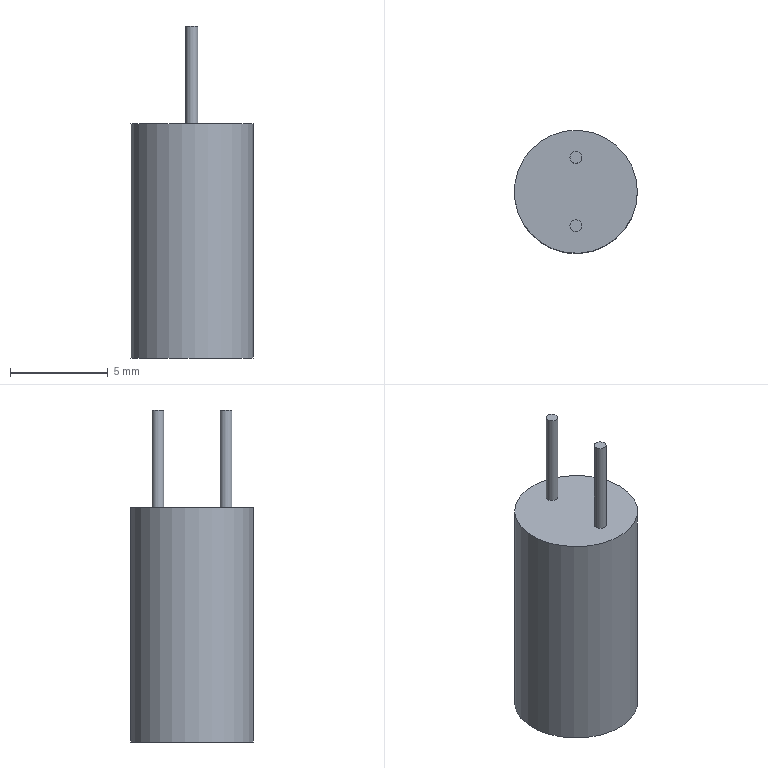Part | STEP file | 118EC225 capacitor | 1 solid | 7 faces | box 6.3 x 6.3 x 17 mm | volume 376.897 mm3 | plane 4 | cylinder 3 | commonest cylinder face diameters 0.6 x2 6.3 x1
STEP:
#1=CARTESIAN_POINT('',(0.,0.,0.));
#2=DIRECTION('',(0.,0.,1.));
#3=DIRECTION('',(1.,0.,0.));
#4=AXIS2_PLACEMENT_3D('',#1,#2,#3);
#5=CARTESIAN_POINT('',(868.15,918.,12.));
#6=VERTEX_POINT('',#5);
#7=CARTESIAN_POINT('',(865.,918.,12.));
#8=DIRECTION('',(0.,0.,1.));
#9=DIRECTION('',(1.,0.,0.));
#10=AXIS2_PLACEMENT_3D('',#7,#8,#9);
#11=CIRCLE('',#10,3.15);
#12=CARTESIAN_POINT('',(865.,918.,12.));
#13=DIRECTION('',(0.,0.,-1.));
#14=DIRECTION('',(-1.,0.,0.));
#15=AXIS2_PLACEMENT_3D('',#12,#13,#14);
#16=CYLINDRICAL_SURFACE('',#15,3.15);
#17=CARTESIAN_POINT('',(9.425,0.));
#18=DIRECTION('',(-1.,0.));
#19=VECTOR('',#18,1.);
#20=LINE('',#17,#19);
#21=(GEOMETRIC_REPRESENTATION_CONTEXT(2)PARAMETRIC_REPRESENTATION_CONTEXT()REPRESENTATION_CONTEXT('',''));
#22=DEFINITIONAL_REPRESENTATION('',(#20),#21);
#23=PCURVE('',#16,#22);
#24=CARTESIAN_POINT('',(865.,918.,12.));
#25=DIRECTION('',(0.,0.,1.));
#26=DIRECTION('',(1.,0.,0.));
#27=AXIS2_PLACEMENT_3D('',#24,#25,#26);
#28=PLANE('',#27);
#29=CARTESIAN_POINT('',(0.,0.));
#30=DIRECTION('',(1.,0.));
#31=AXIS2_PLACEMENT_2D('',#29,#30);
#32=CIRCLE('',#31,3.15);
#33=(GEOMETRIC_REPRESENTATION_CONTEXT(2)PARAMETRIC_REPRESENTATION_CONTEXT()REPRESENTATION_CONTEXT('',''));
#34=DEFINITIONAL_REPRESENTATION('',(#32),#33);
#35=PCURVE('',#28,#34);
#36=SURFACE_CURVE('',#11,(#23,#35),.PCURVE_S1.);
#37=EDGE_CURVE('',#6,#6,#36,.T.);
#38=ORIENTED_EDGE('',*,*,#37,.F.);
#39=CARTESIAN_POINT('',(868.15,918.,0.));
#40=VERTEX_POINT('',#39);
#41=CARTESIAN_POINT('',(868.15,918.,12.));
#42=CARTESIAN_POINT('',(868.15,918.,0.));
#43=B_SPLINE_CURVE_WITH_KNOTS('',1,(#41,#42),.UNSPECIFIED.,.F.,.F.,(2,2),(0.,12.),.PIECEWISE_BEZIER_KNOTS.);
#44=CARTESIAN_POINT('',(9.425,0.));
#45=DIRECTION('',(0.,1.));
#46=VECTOR('',#45,1.);
#47=LINE('',#44,#46);
#48=(GEOMETRIC_REPRESENTATION_CONTEXT(2)PARAMETRIC_REPRESENTATION_CONTEXT()REPRESENTATION_CONTEXT('',''));
#49=DEFINITIONAL_REPRESENTATION('',(#47),#48);
#50=PCURVE('',#16,#49);
#51=CARTESIAN_POINT('',(3.142,0.));
#52=DIRECTION('',(0.,1.));
#53=VECTOR('',#52,1.);
#54=LINE('',#51,#53);
#55=(GEOMETRIC_REPRESENTATION_CONTEXT(2)PARAMETRIC_REPRESENTATION_CONTEXT()REPRESENTATION_CONTEXT('',''));
#56=DEFINITIONAL_REPRESENTATION('',(#54),#55);
#57=PCURVE('',#16,#56);
#58=SEAM_CURVE('',#43,(#50,#57),.PCURVE_S1.);
#59=EDGE_CURVE('',#6,#40,#58,.T.);
#60=ORIENTED_EDGE('',*,*,#59,.T.);
#61=CARTESIAN_POINT('',(865.,918.,0.));
#62=DIRECTION('',(0.,0.,1.));
#63=DIRECTION('',(1.,0.,0.));
#64=AXIS2_PLACEMENT_3D('',#61,#62,#63);
#65=CIRCLE('',#64,3.15);
#66=CARTESIAN_POINT('',(9.425,12.));
#67=DIRECTION('',(-1.,0.));
#68=VECTOR('',#67,1.);
#69=LINE('',#66,#68);
#70=(GEOMETRIC_REPRESENTATION_CONTEXT(2)PARAMETRIC_REPRESENTATION_CONTEXT()REPRESENTATION_CONTEXT('',''));
#71=DEFINITIONAL_REPRESENTATION('',(#69),#70);
#72=PCURVE('',#16,#71);
#73=CARTESIAN_POINT('',(865.,918.,0.));
#74=DIRECTION('',(0.,0.,1.));
#75=DIRECTION('',(1.,0.,0.));
#76=AXIS2_PLACEMENT_3D('',#73,#74,#75);
#77=PLANE('',#76);
#78=CARTESIAN_POINT('',(0.,0.));
#79=DIRECTION('',(1.,0.));
#80=AXIS2_PLACEMENT_2D('',#78,#79);
#81=CIRCLE('',#80,3.15);
#82=(GEOMETRIC_REPRESENTATION_CONTEXT(2)PARAMETRIC_REPRESENTATION_CONTEXT()REPRESENTATION_CONTEXT('',''));
#83=DEFINITIONAL_REPRESENTATION('',(#81),#82);
#84=PCURVE('',#77,#83);
#85=SURFACE_CURVE('',#65,(#72,#84),.PCURVE_S1.);
#86=EDGE_CURVE('',#40,#40,#85,.T.);
#87=ORIENTED_EDGE('',*,*,#86,.T.);
#88=ORIENTED_EDGE('',*,*,#59,.F.);
#89=EDGE_LOOP('',(#38,#60,#87,#88));
#90=FACE_BOUND('',#89,.T.);
#91=ADVANCED_FACE('',(#90),#16,.T.);
#92=CARTESIAN_POINT('',(865.3,916.25,12.));
#93=VERTEX_POINT('',#92);
#94=CARTESIAN_POINT('',(865.,916.25,12.));
#95=DIRECTION('',(0.,0.,1.));
#96=DIRECTION('',(1.,0.,0.));
#97=AXIS2_PLACEMENT_3D('',#94,#95,#96);
#98=CIRCLE('',#97,0.3);
#99=CARTESIAN_POINT('',(0.,-1.75));
#100=DIRECTION('',(1.,0.));
#101=AXIS2_PLACEMENT_2D('',#99,#100);
#102=CIRCLE('',#101,0.3);
#103=(GEOMETRIC_REPRESENTATION_CONTEXT(2)PARAMETRIC_REPRESENTATION_CONTEXT()REPRESENTATION_CONTEXT('',''));
#104=DEFINITIONAL_REPRESENTATION('',(#102),#103);
#105=PCURVE('',#28,#104);
#106=CARTESIAN_POINT('',(865.,916.25,17.));
#107=DIRECTION('',(0.,0.,-1.));
#108=DIRECTION('',(-1.,0.,0.));
#109=AXIS2_PLACEMENT_3D('',#106,#107,#108);
#110=CYLINDRICAL_SURFACE('',#109,0.3);
#111=CARTESIAN_POINT('',(9.425,5.));
#112=DIRECTION('',(-1.,0.));
#113=VECTOR('',#112,1.);
#114=LINE('',#111,#113);
#115=(GEOMETRIC_REPRESENTATION_CONTEXT(2)PARAMETRIC_REPRESENTATION_CONTEXT()REPRESENTATION_CONTEXT('',''));
#116=DEFINITIONAL_REPRESENTATION('',(#114),#115);
#117=PCURVE('',#110,#116);
#118=SURFACE_CURVE('',#98,(#105,#117),.PCURVE_S1.);
#119=EDGE_CURVE('',#93,#93,#118,.T.);
#120=ORIENTED_EDGE('',*,*,#119,.F.);
#121=EDGE_LOOP('',(#120));
#122=FACE_BOUND('',#121,.T.);
#123=CARTESIAN_POINT('',(865.3,919.75,12.));
#124=VERTEX_POINT('',#123);
#125=CARTESIAN_POINT('',(865.,919.75,12.));
#126=DIRECTION('',(0.,0.,1.));
#127=DIRECTION('',(1.,0.,0.));
#128=AXIS2_PLACEMENT_3D('',#125,#126,#127);
#129=CIRCLE('',#128,0.3);
#130=CARTESIAN_POINT('',(0.,1.75));
#131=DIRECTION('',(1.,0.));
#132=AXIS2_PLACEMENT_2D('',#130,#131);
#133=CIRCLE('',#132,0.3);
#134=(GEOMETRIC_REPRESENTATION_CONTEXT(2)PARAMETRIC_REPRESENTATION_CONTEXT()REPRESENTATION_CONTEXT('',''));
#135=DEFINITIONAL_REPRESENTATION('',(#133),#134);
#136=PCURVE('',#28,#135);
#137=CARTESIAN_POINT('',(865.,919.75,17.));
#138=DIRECTION('',(0.,0.,-1.));
#139=DIRECTION('',(-1.,0.,0.));
#140=AXIS2_PLACEMENT_3D('',#137,#138,#139);
#141=CYLINDRICAL_SURFACE('',#140,0.3);
#142=CARTESIAN_POINT('',(9.425,5.));
#143=DIRECTION('',(-1.,0.));
#144=VECTOR('',#143,1.);
#145=LINE('',#142,#144);
#146=(GEOMETRIC_REPRESENTATION_CONTEXT(2)PARAMETRIC_REPRESENTATION_CONTEXT()REPRESENTATION_CONTEXT('',''));
#147=DEFINITIONAL_REPRESENTATION('',(#145),#146);
#148=PCURVE('',#141,#147);
#149=SURFACE_CURVE('',#129,(#136,#148),.PCURVE_S1.);
#150=EDGE_CURVE('',#124,#124,#149,.T.);
#151=ORIENTED_EDGE('',*,*,#150,.F.);
#152=EDGE_LOOP('',(#151));
#153=FACE_BOUND('',#152,.T.);
#154=ORIENTED_EDGE('',*,*,#37,.T.);
#155=EDGE_LOOP('',(#154));
#156=FACE_BOUND('',#155,.T.);
#157=ADVANCED_FACE('',(#122,#153,#156),#28,.T.);
#158=ORIENTED_EDGE('',*,*,#86,.F.);
#159=EDGE_LOOP('',(#158));
#160=FACE_BOUND('',#159,.T.);
#161=ADVANCED_FACE('',(#160),#77,.F.);
#162=CARTESIAN_POINT('',(865.3,919.75,17.));
#163=VERTEX_POINT('',#162);
#164=CARTESIAN_POINT('',(865.,919.75,17.));
#165=DIRECTION('',(0.,0.,1.));
#166=DIRECTION('',(1.,0.,0.));
#167=AXIS2_PLACEMENT_3D('',#164,#165,#166);
#168=CIRCLE('',#167,0.3);
#169=CARTESIAN_POINT('',(9.425,0.));
#170=DIRECTION('',(-1.,0.));
#171=VECTOR('',#170,1.);
#172=LINE('',#169,#171);
#173=(GEOMETRIC_REPRESENTATION_CONTEXT(2)PARAMETRIC_REPRESENTATION_CONTEXT()REPRESENTATION_CONTEXT('',''));
#174=DEFINITIONAL_REPRESENTATION('',(#172),#173);
#175=PCURVE('',#141,#174);
#176=CARTESIAN_POINT('',(865.,919.75,17.));
#177=DIRECTION('',(0.,0.,1.));
#178=DIRECTION('',(1.,0.,0.));
#179=AXIS2_PLACEMENT_3D('',#176,#177,#178);
#180=PLANE('',#179);
#181=CARTESIAN_POINT('',(0.,0.));
#182=DIRECTION('',(1.,0.));
#183=AXIS2_PLACEMENT_2D('',#181,#182);
#184=CIRCLE('',#183,0.3);
#185=(GEOMETRIC_REPRESENTATION_CONTEXT(2)PARAMETRIC_REPRESENTATION_CONTEXT()REPRESENTATION_CONTEXT('',''));
#186=DEFINITIONAL_REPRESENTATION('',(#184),#185);
#187=PCURVE('',#180,#186);
#188=SURFACE_CURVE('',#168,(#175,#187),.PCURVE_S1.);
#189=EDGE_CURVE('',#163,#163,#188,.T.);
#190=ORIENTED_EDGE('',*,*,#189,.F.);
#191=CARTESIAN_POINT('',(865.3,919.75,17.));
#192=CARTESIAN_POINT('',(865.3,919.75,12.));
#193=B_SPLINE_CURVE_WITH_KNOTS('',1,(#191,#192),.UNSPECIFIED.,.F.,.F.,(2,2),(0.,5.),.PIECEWISE_BEZIER_KNOTS.);
#194=CARTESIAN_POINT('',(9.425,0.));
#195=DIRECTION('',(0.,1.));
#196=VECTOR('',#195,1.);
#197=LINE('',#194,#196);
#198=(GEOMETRIC_REPRESENTATION_CONTEXT(2)PARAMETRIC_REPRESENTATION_CONTEXT()REPRESENTATION_CONTEXT('',''));
#199=DEFINITIONAL_REPRESENTATION('',(#197),#198);
#200=PCURVE('',#141,#199);
#201=CARTESIAN_POINT('',(3.142,0.));
#202=DIRECTION('',(0.,1.));
#203=VECTOR('',#202,1.);
#204=LINE('',#201,#203);
#205=(GEOMETRIC_REPRESENTATION_CONTEXT(2)PARAMETRIC_REPRESENTATION_CONTEXT()REPRESENTATION_CONTEXT('',''));
#206=DEFINITIONAL_REPRESENTATION('',(#204),#205);
#207=PCURVE('',#141,#206);
#208=SEAM_CURVE('',#193,(#200,#207),.PCURVE_S1.);
#209=EDGE_CURVE('',#163,#124,#208,.T.);
#210=ORIENTED_EDGE('',*,*,#209,.T.);
#211=ORIENTED_EDGE('',*,*,#150,.T.);
#212=ORIENTED_EDGE('',*,*,#209,.F.);
#213=EDGE_LOOP('',(#190,#210,#211,#212));
#214=FACE_BOUND('',#213,.T.);
#215=ADVANCED_FACE('',(#214),#141,.T.);
#216=ORIENTED_EDGE('',*,*,#189,.T.);
#217=EDGE_LOOP('',(#216));
#218=FACE_BOUND('',#217,.T.);
#219=ADVANCED_FACE('',(#218),#180,.T.);
#220=CARTESIAN_POINT('',(865.3,916.25,17.));
#221=VERTEX_POINT('',#220);
#222=CARTESIAN_POINT('',(865.,916.25,17.));
#223=DIRECTION('',(0.,0.,-1.));
#224=DIRECTION('',(1.,0.,0.));
#225=AXIS2_PLACEMENT_3D('',#222,#223,#224);
#226=CIRCLE('',#225,0.3);
#227=CARTESIAN_POINT('',(3.142,0.));
#228=DIRECTION('',(1.,0.));
#229=VECTOR('',#228,1.);
#230=LINE('',#227,#229);
#231=(GEOMETRIC_REPRESENTATION_CONTEXT(2)PARAMETRIC_REPRESENTATION_CONTEXT()REPRESENTATION_CONTEXT('',''));
#232=DEFINITIONAL_REPRESENTATION('',(#230),#231);
#233=PCURVE('',#110,#232);
#234=CARTESIAN_POINT('',(865.,916.25,17.));
#235=DIRECTION('',(0.,0.,-1.));
#236=DIRECTION('',(-1.,0.,0.));
#237=AXIS2_PLACEMENT_3D('',#234,#235,#236);
#238=PLANE('',#237);
#239=CARTESIAN_POINT('',(0.,0.));
#240=DIRECTION('',(-1.,0.));
#241=AXIS2_PLACEMENT_2D('',#239,#240);
#242=CIRCLE('',#241,0.3);
#243=(GEOMETRIC_REPRESENTATION_CONTEXT(2)PARAMETRIC_REPRESENTATION_CONTEXT()REPRESENTATION_CONTEXT('',''));
#244=DEFINITIONAL_REPRESENTATION('',(#242),#243);
#245=PCURVE('',#238,#244);
#246=SURFACE_CURVE('',#226,(#233,#245),.PCURVE_S1.);
#247=EDGE_CURVE('',#221,#221,#246,.T.);
#248=ORIENTED_EDGE('',*,*,#247,.T.);
#249=CARTESIAN_POINT('',(865.3,916.25,17.));
#250=CARTESIAN_POINT('',(865.3,916.25,12.));
#251=B_SPLINE_CURVE_WITH_KNOTS('',1,(#249,#250),.UNSPECIFIED.,.F.,.F.,(2,2),(0.,5.),.PIECEWISE_BEZIER_KNOTS.);
#252=CARTESIAN_POINT('',(9.425,0.));
#253=DIRECTION('',(0.,1.));
#254=VECTOR('',#253,1.);
#255=LINE('',#252,#254);
#256=(GEOMETRIC_REPRESENTATION_CONTEXT(2)PARAMETRIC_REPRESENTATION_CONTEXT()REPRESENTATION_CONTEXT('',''));
#257=DEFINITIONAL_REPRESENTATION('',(#255),#256);
#258=PCURVE('',#110,#257);
#259=CARTESIAN_POINT('',(3.142,0.));
#260=DIRECTION('',(0.,1.));
#261=VECTOR('',#260,1.);
#262=LINE('',#259,#261);
#263=(GEOMETRIC_REPRESENTATION_CONTEXT(2)PARAMETRIC_REPRESENTATION_CONTEXT()REPRESENTATION_CONTEXT('',''));
#264=DEFINITIONAL_REPRESENTATION('',(#262),#263);
#265=PCURVE('',#110,#264);
#266=SEAM_CURVE('',#251,(#258,#265),.PCURVE_S1.);
#267=EDGE_CURVE('',#221,#93,#266,.T.);
#268=ORIENTED_EDGE('',*,*,#267,.T.);
#269=ORIENTED_EDGE('',*,*,#119,.T.);
#270=ORIENTED_EDGE('',*,*,#267,.F.);
#271=EDGE_LOOP('',(#248,#268,#269,#270));
#272=FACE_BOUND('',#271,.T.);
#273=ADVANCED_FACE('',(#272),#110,.T.);
#274=ORIENTED_EDGE('',*,*,#247,.F.);
#275=EDGE_LOOP('',(#274));
#276=FACE_BOUND('',#275,.T.);
#277=ADVANCED_FACE('',(#276),#238,.F.);
#278=CLOSED_SHELL('',(#91,#157,#161,#215,#219,#273,#277));
#279=MANIFOLD_SOLID_BREP('',#278);
#280=(LENGTH_UNIT()NAMED_UNIT(*)SI_UNIT(.MILLI.,.METRE.));
#281=UNCERTAINTY_MEASURE_WITH_UNIT(LENGTH_MEASURE(0.00001),#280,'','');
#282=(NAMED_UNIT(*)PLANE_ANGLE_UNIT()SI_UNIT($,.RADIAN.));
#283=(NAMED_UNIT(*)SI_UNIT($,.STERADIAN.)SOLID_ANGLE_UNIT());
#284=(GEOMETRIC_REPRESENTATION_CONTEXT(3)GLOBAL_UNCERTAINTY_ASSIGNED_CONTEXT((#281))GLOBAL_UNIT_ASSIGNED_CONTEXT((#280,#282,#283))REPRESENTATION_CONTEXT('',''));
#285=ADVANCED_BREP_SHAPE_REPRESENTATION('',(#4,#279),#284);